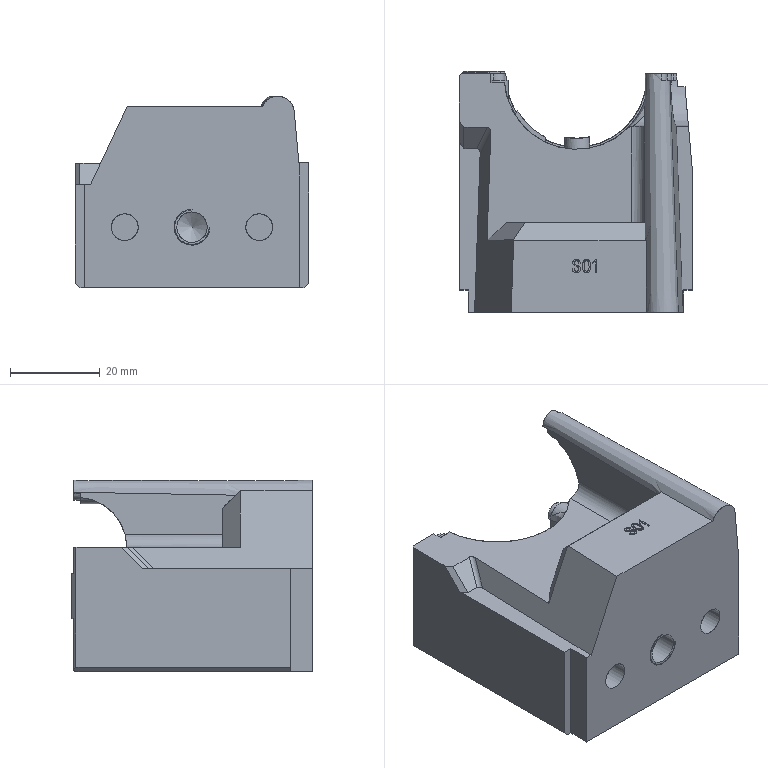NC program | PowerMill | posted with a generic post | part box 52 x 53.756 x 42.711 mm
Whole program:
%
O0001
N104 ( POWERMILL CB  : 2026004.0)
N105 ( POST VER      : 2026.0.0.5161)
N106 ( OPTION FILE   : FANUC)
N107 ( OUTPUT WORKPLANE : 1)
N108 (  )
N109 ( TOOL LIST )
N110 (--------------------------------)
N111 ( NO. | ID | DIA.| TIP RAD|LENGTH)
N112 (--------------------------------)
N113 (    1|D8_3| 8.0 |  0.0   | 99.0 )
N114 (--------------------------------)
N115 (  )
N116 ( NUMBER OF TOOLPATHS: 2.0 )
N117 ( ESTIMATED PROGRAM DURATION: 0 HOURS 2 MIN 27 SEC)
N118 (  )
N119 G00 G21 G80 G40 G17
N120 G90
N121 G54
N122 G53 Z0.0
N123 (---------------)
N124 ( START TOOLPATH : 04精光-D8-偏置平坦面 )
N125 (---------------)
N126 ( TOOL NO.    :1 )
N127 ( TOOL TYPE   : ENDMILL)
N128 ( TOOL ID     : D8_3)
N129 ( TOOL DIA    : 8.0 LENGTH 99.0)
N130 T1
N131 M6
N132 S3500 M03
N133 G00 G90 X-27.783 Y-7.9491
N134 G43 Z20.0 H1
N135
N136 G05 P10000 R8
N137 Z-2.0
N138 G01 Z-5.0 F480.0
N139 X-26.3387 Y-3.984 F800.0
N140 G03 X-26.0 Y-3.9983 I0.3387 J3.9841
N141 G01 X-25.2845
N142 G02 X-28.1881 Y-0.3178 I1.2821 J3.997
N143 G02 X-28.2001 Y0.2956 I6.337 J0.4306
N144 G01 Y44.8679
N145 G02 X-27.9783 Y46.1846 I4.0947 J-0.0127
N146 G00 Z5.0625
N147 G01 X33.9831 Y-1.6873 F10000.0
N148 G00 Z-2.0
N149 G01 Z-5.0 F480.0
N150 X29.9838 Y-0.3406 F800.0
N151 G03 X29.9983 Y0.0 I-3.9839 J0.3406
N152 G01 Y42.71
N153 G03 X27.9782 Y46.1846 I-3.9983 J0.0
N154 G02 X28.2001 Y44.8679 I-3.8786 J-1.3304
N155 G01 Y0.2956
N156 G02 X28.1333 Y-0.7465 I-4.9114 J-0.2084
N157 G02 X25.2845 Y-3.9983 I-4.1307 J0.7449
N158 G00 Z20.0
N159 G05 P0
N160 (---------------)
N161 ( END TOOLPATH : 04精光-D8-偏置平坦面 )
N162 (---------------)
N163 ( START TOOLPATH : 03精光-D8-等高 )
N164 (---------------)
N165 S5500 M03
N166 G00 X28.2044 Y43.463 Z20.0
N167 G05 P10000 R8
N168 Z2.9018
N169 G01 Z-0.0982 F1200.0
N170 G03 X27.99 Y42.663 I1.3856 J-0.8 F2000.0
N171 G01 Y0.047
N172 G03 X28.2044 Y-0.753 I1.6 J0.0
N173 G01 X28.2217 Y-0.7831 Z-0.1125
N174 X28.2289 Y-0.7955 Z-0.1472
N175 X28.2217 Y-0.7831 Z-0.1819
N176 X28.2044 Y-0.753 Z-0.1963
N177 G02 X27.99 Y0.047 I1.3856 J0.8
N178 G01 Y42.663
N179 G02 X28.2044 Y43.463 I1.6 J0.0
N180 G01 X28.2217 Y43.4931 Z-0.2107
N181 X28.2289 Y43.5055 Z-0.2454
N182 X28.2217 Y43.4931 Z-0.2801
N183 X28.2044 Y43.463 Z-0.2945
N184 G03 X27.99 Y42.663 I1.3856 J-0.8
N185 G01 Y0.047
N186 G03 X28.2044 Y-0.753 I1.6 J0.0
N187 G01 X28.2217 Y-0.7831 Z-0.3088
N188 X28.2289 Y-0.7955 Z-0.3435
N189 X28.2217 Y-0.7831 Z-0.3783
N190 X28.2044 Y-0.753 Z-0.3926
N191 G02 X27.99 Y0.047 I1.3856 J0.8
N192 G01 Y42.663
N193 G02 X28.2044 Y43.463 I1.6 J0.0
N194 G01 X28.2217 Y43.4931 Z-0.407
N195 X28.2289 Y43.5055 Z-0.4417
N196 X28.2217 Y43.4931 Z-0.4764
N197 X28.2044 Y43.463 Z-0.4908
N198 G03 X27.99 Y42.663 I1.3856 J-0.8
N199 G01 Y0.047
N200 G03 X28.2044 Y-0.753 I1.6 J0.0
N201 G01 X28.2217 Y-0.7831 Z-0.5052
N202 X28.2289 Y-0.7955 Z-0.5399
N203 X28.2217 Y-0.7831 Z-0.5746
N204 X28.2044 Y-0.753 Z-0.5889
N205 G02 X27.99 Y0.047 I1.3856 J0.8
N206 G01 Y42.663
N207 G02 X28.2044 Y43.463 I1.6 J0.0
N208 G01 X28.2217 Y43.4931 Z-0.6033
N209 X28.2289 Y43.5055 Z-0.638
N210 X28.2217 Y43.4931 Z-0.6727
N211 X28.2044 Y43.463 Z-0.6871
N212 G03 X27.99 Y42.663 I1.3856 J-0.8
N213 G01 Y0.047
N214 G03 X28.2044 Y-0.753 I1.6 J0.0
N215 G01 X28.2217 Y-0.7831 Z-0.7015
N216 X28.2289 Y-0.7955 Z-0.7362
N217 X28.2217 Y-0.7831 Z-0.7709
N218 X28.2044 Y-0.753 Z-0.7853
N219 G02 X27.99 Y0.047 I1.3856 J0.8
N220 G01 Y42.663
N221 G02 X28.2044 Y43.463 I1.6 J0.0
N222 G01 X28.2217 Y43.4931 Z-0.7996
N223 X28.2289 Y43.5055 Z-0.8343
N224 X28.2217 Y43.4931 Z-0.869
N225 X28.2044 Y43.463 Z-0.8834
N226 G03 X27.99 Y42.663 I1.3856 J-0.8
N227 G01 Y0.047
N228 G03 X28.2044 Y-0.753 I1.6 J0.0
N229 G01 X28.2217 Y-0.7831 Z-0.8978
N230 X28.2289 Y-0.7955 Z-0.9325
N231 X28.2217 Y-0.7831 Z-0.9672
N232 X28.2044 Y-0.753 Z-0.9816
N233 G02 X27.99 Y0.047 I1.3856 J0.8
N234 G01 Y42.663
N235 G02 X28.2044 Y43.463 I1.6 J0.0
N236 G01 X28.2217 Y43.4931 Z-0.9959
N237 X28.2289 Y43.5055 Z-1.0306
N238 X28.2217 Y43.4931 Z-1.0654
N239 X28.2044 Y43.463 Z-1.0797
N240 G03 X27.99 Y42.663 I1.3856 J-0.8
N241 G01 Y0.047
N242 G03 X28.2044 Y-0.753 I1.6 J0.0
N243 G01 X28.2217 Y-0.7831 Z-1.0941
N244 X28.2289 Y-0.7955 Z-1.1288
N245 X28.2217 Y-0.7831 Z-1.1635
N246 X28.2044 Y-0.753 Z-1.1779
N247 G02 X27.99 Y0.047 I1.3856 J0.8
N248 G01 Y42.663
N249 G02 X28.2044 Y43.463 I1.6 J0.0
N250 G01 X28.2217 Y43.4931 Z-1.1923
N251 X28.2289 Y43.5055 Z-1.227
N252 X28.2217 Y43.4931 Z-1.2617
N253 X28.2044 Y43.463 Z-1.276
N254 G03 X27.99 Y42.663 I1.3856 J-0.8
N255 G01 Y0.047
N256 G03 X28.2044 Y-0.753 I1.6 J0.0
N257 G01 X28.2217 Y-0.7831 Z-1.2904
N258 X28.2289 Y-0.7955 Z-1.3251
N259 X28.2217 Y-0.7831 Z-1.3598
N260 X28.2044 Y-0.753 Z-1.3742
N261 G02 X27.99 Y0.047 I1.3856 J0.8
N262 G01 Y42.663
N263 G02 X28.2044 Y43.463 I1.6 J0.0
N264 G01 X28.2217 Y43.4931 Z-1.3886
N265 X28.2289 Y43.5055 Z-1.4233
N266 X28.2217 Y43.4931 Z-1.458
N267 X28.2044 Y43.463 Z-1.4724
N268 G03 X27.99 Y42.663 I1.3856 J-0.8
N269 G01 Y0.047
N270 G03 X28.2044 Y-0.753 I1.6 J0.0
N271 G01 X28.2217 Y-0.7831 Z-1.4867
N272 X28.2289 Y-0.7955 Z-1.5214
N273 X28.2217 Y-0.7831 Z-1.5561
N274 X28.2044 Y-0.753 Z-1.5705
N275 G02 X27.99 Y0.047 I1.3856 J0.8
N276 G01 Y42.663
N277 G02 X28.2044 Y43.463 I1.6 J0.0
N278 G01 X28.2217 Y43.4931 Z-1.5849
N279 X28.2289 Y43.5055 Z-1.6196
N280 X28.2217 Y43.4931 Z-1.6543
N281 X28.2044 Y43.463 Z-1.6687
N282 G03 X27.99 Y42.663 I1.3856 J-0.8
N283 G01 Y0.047
N284 G03 X28.2044 Y-0.753 I1.6 J0.0
N285 G01 X28.2217 Y-0.7831 Z-1.683
N286 X28.2289 Y-0.7955 Z-1.7177
N287 X28.2217 Y-0.7831 Z-1.7524
N288 X28.2044 Y-0.753 Z-1.7668
N289 G02 X27.99 Y0.047 I1.3856 J0.8
N290 G01 Y42.663
N291 G02 X28.2044 Y43.463 I1.6 J0.0
N292 G01 X28.2217 Y43.4931 Z-1.7812
N293 X28.2289 Y43.5055 Z-1.8159
N294 X28.2217 Y43.4931 Z-1.8506
N295 X28.2044 Y43.463 Z-1.865
N296 G03 X27.99 Y42.663 I1.3856 J-0.8
N297 G01 Y0.047
N298 G03 X28.2044 Y-0.753 I1.6 J0.0
N299 G01 X28.2217 Y-0.7831 Z-1.8794
N300 X28.2289 Y-0.7955 Z-1.9141
N301 X28.2217 Y-0.7831 Z-1.9488
N302 X28.2044 Y-0.753 Z-1.9631
N303 G02 X27.99 Y0.047 I1.3856 J0.8
N304 G01 Y42.663
N305 G02 X28.2044 Y43.463 I1.6 J0.0
N306 G01 X28.2217 Y43.4931 Z-1.9775
N307 X28.2289 Y43.5055 Z-2.0122
N308 X28.2217 Y43.4931 Z-2.0469
N309 X28.2044 Y43.463 Z-2.0613
N310 G03 X27.99 Y42.663 I1.3856 J-0.8
N311 G01 Y0.047
N312 G03 X28.2044 Y-0.753 I1.6 J0.0
N313 G01 X28.2217 Y-0.7831 Z-2.0757
N314 X28.2289 Y-0.7955 Z-2.1104
N315 X28.2217 Y-0.7831 Z-2.1451
N316 X28.2044 Y-0.753 Z-2.1595
N317 G02 X27.99 Y0.047 I1.3856 J0.8
N318 G01 Y42.663
N319 G02 X28.2044 Y43.463 I1.6 J0.0
N320 G01 X28.2217 Y43.4931 Z-2.1738
N321 X28.2289 Y43.5055 Z-2.2085
N322 X28.2217 Y43.4931 Z-2.2432
N323 X28.2044 Y43.463 Z-2.2576
N324 G03 X27.99 Y42.663 I1.3856 J-0.8
N325 G01 Y0.047
N326 G03 X28.2044 Y-0.753 I1.6 J0.0
N327 G01 X28.2217 Y-0.7831 Z-2.272
N328 X28.2289 Y-0.7955 Z-2.3067
N329 X28.2217 Y-0.7831 Z-2.3414
N330 X28.2044 Y-0.753 Z-2.3558
N331 G02 X27.99 Y0.047 I1.3856 J0.8
N332 G01 Y42.663
N333 G02 X28.2044 Y43.463 I1.6 J0.0
N334 G01 X28.2217 Y43.4931 Z-2.3701
N335 X28.2289 Y43.5055 Z-2.4048
N336 X28.2217 Y43.4931 Z-2.4395
N337 X28.2044 Y43.463 Z-2.4539
N338 G03 X27.99 Y42.663 I1.3856 J-0.8
N339 G01 Y0.047
N340 G03 X28.2044 Y-0.753 I1.6 J0.0
N341 G01 X28.2217 Y-0.7831 Z-2.4683
N342 X28.2289 Y-0.7955 Z-2.503
N343 X28.2217 Y-0.7831 Z-2.5377
N344 X28.2044 Y-0.753 Z-2.5521
N345 G02 X27.99 Y0.047 I1.3856 J0.8
N346 G01 Y42.663
N347 G02 X28.2044 Y43.463 I1.6 J0.0
N348 G01 X28.2217 Y43.4931 Z-2.5665
N349 X28.2289 Y43.5055 Z-2.6012
N350 X28.2217 Y43.4931 Z-2.6359
N351 X28.2044 Y43.463 Z-2.6502
N352 G03 X27.99 Y42.663 I1.3856 J-0.8
N353 G01 Y0.047
N354 G03 X28.2044 Y-0.753 I1.6 J0.0
N355 G01 X28.2217 Y-0.7831 Z-2.6646
N356 X28.2289 Y-0.7955 Z-2.6993
N357 X28.2217 Y-0.7831 Z-2.734
N358 X28.2044 Y-0.753 Z-2.7484
N359 G02 X27.99 Y0.047 I1.3856 J0.8
N360 G01 Y42.663
N361 G02 X28.2044 Y43.463 I1.6 J0.0
N362 G01 X28.2217 Y43.4931 Z-2.7628
N363 X28.2289 Y43.5055 Z-2.7975
N364 X28.2217 Y43.4931 Z-2.8322
N365 X28.2044 Y43.463 Z-2.8465
N366 G03 X27.99 Y42.663 I1.3856 J-0.8
N367 G01 Y0.047
N368 G03 X28.2044 Y-0.753 I1.6 J0.0
N369 G01 X28.2217 Y-0.7831 Z-2.8609
N370 X28.2289 Y-0.7955 Z-2.8956
N371 X28.2217 Y-0.7831 Z-2.9303
N372 X28.2044 Y-0.753 Z-2.9447
N373 G02 X27.99 Y0.047 I1.3856 J0.8
N374 G01 Y42.663
N375 G02 X28.2044 Y43.463 I1.6 J0.0
N376 G01 X28.2217 Y43.4931 Z-2.9591
N377 X28.2289 Y43.5055 Z-2.9938
N378 X28.2217 Y43.4931 Z-3.0285
N379 X28.2044 Y43.463 Z-3.0429
N380 G03 X27.99 Y42.663 I1.3856 J-0.8
N381 G01 Y0.047
N382 G03 X28.2044 Y-0.753 I1.6 J0.0
N383 G01 X28.2217 Y-0.7831 Z-3.0572
N384 X28.2289 Y-0.7955 Z-3.0919
N385 X28.2217 Y-0.7831 Z-3.1266
N386 X28.2044 Y-0.753 Z-3.141
N387 G02 X27.99 Y0.047 I1.3856 J0.8
N388 G01 Y42.663
N389 G02 X28.2044 Y43.463 I1.6 J0.0
N390 G01 X28.2217 Y43.4931 Z-3.1554
N391 X28.2289 Y43.5055 Z-3.1901
N392 X28.2217 Y43.4931 Z-3.2248
N393 X28.2044 Y43.463 Z-3.2392
N394 G03 X27.99 Y42.663 I1.3856 J-0.8
N395 G01 Y0.047
N396 G03 X28.2044 Y-0.753 I1.6 J0.0
N397 G01 X28.2217 Y-0.7831 Z-3.2536
N398 X28.2289 Y-0.7955 Z-3.2883
N399 X28.2217 Y-0.7831 Z-3.323
N400 X28.2044 Y-0.753 Z-3.3373
N401 G02 X27.99 Y0.047 I1.3856 J0.8
N402 G01 Y42.663
N403 G02 X28.2044 Y43.463 I1.6 J0.0
N404 G01 X28.2217 Y43.4931 Z-3.3517
N405 X28.2289 Y43.5055 Z-3.3864
N406 X28.2217 Y43.4931 Z-3.4211
N407 X28.2044 Y43.463 Z-3.4355
N408 G03 X27.99 Y42.663 I1.3856 J-0.8
N409 G01 Y0.047
N410 G03 X28.2044 Y-0.753 I1.6 J0.0
N411 G01 X28.2217 Y-0.7831 Z-3.4499
N412 X28.2289 Y-0.7955 Z-3.4846
N413 X28.2217 Y-0.7831 Z-3.5193
N414 X28.2044 Y-0.753 Z-3.5336
N415 G02 X27.99 Y0.047 I1.3856 J0.8
N416 G01 Y42.663
N417 G02 X28.2044 Y43.463 I1.6 J0.0
N418 G01 X28.2217 Y43.4931 Z-3.548
N419 X28.2289 Y43.5055 Z-3.5827
N420 X28.2217 Y43.4931 Z-3.6174
N421 X28.2044 Y43.463 Z-3.6318
N422 G03 X27.99 Y42.663 I1.3856 J-0.8
N423 G01 Y0.047
N424 G03 X28.2044 Y-0.753 I1.6 J0.0
N425 G01 X28.2217 Y-0.7831 Z-3.6462
N426 X28.2289 Y-0.7955 Z-3.6809
N427 X28.2217 Y-0.7831 Z-3.7156
N428 X28.2044 Y-0.753 Z-3.73
N429 G02 X27.99 Y0.047 I1.3856 J0.8
N430 G01 Y42.663
N431 G02 X28.2044 Y43.463 I1.6 J0.0
N432 G01 X28.2217 Y43.4931 Z-3.7443
N433 X28.2289 Y43.5055 Z-3.779
N434 X28.2217 Y43.4931 Z-3.8137
N435 X28.2044 Y43.463 Z-3.8281
N436 G03 X27.99 Y42.663 I1.3856 J-0.8
N437 G01 Y0.047
N438 G03 X28.2044 Y-0.753 I1.6 J0.0
N439 G01 X28.2217 Y-0.7831 Z-3.8425
N440 X28.2289 Y-0.7955 Z-3.8772
N441 X28.2217 Y-0.7831 Z-3.9119
N442 X28.2044 Y-0.753 Z-3.9263
N443 G02 X27.99 Y0.047 I1.3856 J0.8
N444 G01 Y42.663
N445 G02 X28.2044 Y43.463 I1.6 J0.0
N446 G01 X28.2217 Y43.4931 Z-3.9406
N447 X28.2289 Y43.5055 Z-3.9754
N448 X28.2217 Y43.4931 Z-4.0101
N449 X28.2044 Y43.463 Z-4.0244
N450 G03 X27.99 Y42.663 I1.3856 J-0.8
N451 G01 Y0.047
N452 G03 X28.2044 Y-0.753 I1.6 J0.0
N453 G01 X28.2217 Y-0.7831 Z-4.0388
N454 X28.2289 Y-0.7955 Z-4.0735
N455 X28.2217 Y-0.7831 Z-4.1082
N456 X28.2044 Y-0.753 Z-4.1226
N457 G02 X27.99 Y0.047 I1.3856 J0.8
N458 G01 Y42.663
N459 G02 X28.2044 Y43.463 I1.6 J0.0
N460 G01 X28.2217 Y43.4931 Z-4.137
N461 X28.2289 Y43.5055 Z-4.1717
N462 X28.2217 Y43.4931 Z-4.2064
N463 X28.2044 Y43.463 Z-4.2207
N464 G03 X27.99 Y42.663 I1.3856 J-0.8
N465 G01 Y0.047
N466 G03 X28.2044 Y-0.753 I1.6 J0.0
N467 G01 X28.2217 Y-0.7831 Z-4.2351
N468 X28.2289 Y-0.7955 Z-4.2698
N469 X28.2217 Y-0.7831 Z-4.3045
N470 X28.2044 Y-0.753 Z-4.3189
N471 G02 X27.99 Y0.047 I1.3856 J0.8
N472 G01 Y42.663
N473 G02 X28.2044 Y43.463 I1.6 J0.0
N474 G01 X28.2217 Y43.4931 Z-4.3333
N475 X28.2289 Y43.5055 Z-4.368
N476 X28.2217 Y43.4931 Z-4.4027
N477 X28.2044 Y43.463 Z-4.4171
N478 G03 X27.99 Y42.663 I1.3856 J-0.8
N479 G01 Y0.047
N480 G03 X28.2044 Y-0.753 I1.6 J0.0
N481 G01 X28.2217 Y-0.7831 Z-4.4314
N482 X28.2289 Y-0.7955 Z-4.4661
N483 X28.2217 Y-0.7831 Z-4.5008
N484 X28.2044 Y-0.753 Z-4.5152
N485 G02 X27.99 Y0.047 I1.3856 J0.8
N486 G01 Y42.663
N487 G02 X28.2044 Y43.463 I1.6 J0.0
N488 G01 X28.2217 Y43.4931 Z-4.5296
N489 X28.2289 Y43.5055 Z-4.5643
N490 X28.2217 Y43.4931 Z-4.599
N491 X28.2044 Y43.463 Z-4.6134
N492 G03 X27.99 Y42.663 I1.3856 J-0.8
N493 G01 Y0.047
N494 G03 X28.2044 Y-0.753 I1.6 J0.0
N495 G01 X28.2217 Y-0.7831 Z-4.6277
N496 X28.2289 Y-0.7955 Z-4.6625
N497 X28.2217 Y-0.7831 Z-4.6972
N498 X28.2044 Y-0.753 Z-4.7115
N499 G02 X27.99 Y0.047 I1.3856 J0.8
N500 G01 Y42.663
N501 G02 X28.2044 Y43.463 I1.6 J0.0
N502 G01 X28.2217 Y43.4931 Z-4.7259
N503 X28.2289 Y43.5055 Z-4.7606
N504 X28.2217 Y43.4931 Z-4.7953
N505 X28.2044 Y43.463 Z-4.8097
N506 G03 X27.99 Y42.663 I1.3856 J-0.8
N507 G01 Y0.047
N508 G03 X28.2044 Y-0.753 I1.6 J0.0
N509 G01 X28.2217 Y-0.7831 Z-4.8241
N510 X28.2289 Y-0.7955 Z-4.8588
N511 X28.2217 Y-0.7831 Z-4.8935
N512 X28.2044 Y-0.753 Z-4.9078
N513 G02 X27.99 Y0.047 I1.3856 J0.8
N514 G01 Y42.663
N515 G02 X28.2044 Y43.463 I1.6 J0.0
N516 G00 Z5.0391
N517 G01 X-28.2044 Y-0.753 F10000.0
N518 G00 Z2.9018
N519 G01 Z-0.0982 F1200.0
N520 G03 X-27.99 Y0.047 I-1.3856 J0.8 F2000.0
N521 G01 Y42.663
N522 G03 X-28.2044 Y43.463 I-1.6 J0.0
N523 G01 X-28.2217 Y43.4931 Z-0.1125
N524 X-28.2289 Y43.5055 Z-0.1472
N525 X-28.2217 Y43.4931 Z-0.1819
N526 X-28.2044 Y43.463 Z-0.1963
N527 G02 X-27.99 Y42.663 I-1.3856 J-0.8
N528 G01 Y0.047
N529 G02 X-28.2044 Y-0.753 I-1.6 J0.0
N530 G01 X-28.2217 Y-0.7831 Z-0.2107
N531 X-28.2289 Y-0.7955 Z-0.2454
N532 X-28.2217 Y-0.7831 Z-0.2801
N533 X-28.2044 Y-0.753 Z-0.2945
N534 G03 X-27.99 Y0.047 I-1.3856 J0.8
N535 G01 Y42.663
N536 G03 X-28.2044 Y43.463 I-1.6 J0.0
N537 G01 X-28.2217 Y43.4931 Z-0.3088
N538 X-28.2289 Y43.5055 Z-0.3435
N539 X-28.2217 Y43.4931 Z-0.3783
N540 X-28.2044 Y43.463 Z-0.3926
N541 G02 X-27.99 Y42.663 I-1.3856 J-0.8
N542 G01 Y0.047
N543 G02 X-28.2044 Y-0.753 I-1.6 J0.0
N544 G01 X-28.2217 Y-0.7831 Z-0.407
N545 X-28.2289 Y-0.7955 Z-0.4417
N546 X-28.2217 Y-0.7831 Z-0.4764
N547 X-28.2044 Y-0.753 Z-0.4908
N548 G03 X-27.99 Y0.047 I-1.3856 J0.8
N549 G01 Y42.663
N550 G03 X-28.2044 Y43.463 I-1.6 J0.0
N551 G01 X-28.2217 Y43.4931 Z-0.5052
N552 X-28.2289 Y43.5055 Z-0.5399
N553 X-28.2217 Y43.4931 Z-0.5746
N554 X-28.2044 Y43.463 Z-0.5889
N555 G02 X-27.99 Y42.663 I-1.3856 J-0.8
N556 G01 Y0.047
N557 G02 X-28.2044 Y-0.753 I-1.6 J0.0
N558 G01 X-28.2217 Y-0.7831 Z-0.6033
N559 X-28.2289 Y-0.7955 Z-0.638
N560 X-28.2217 Y-0.7831 Z-0.6727
N561 X-28.2044 Y-0.753 Z-0.6871
N562 G03 X-27.99 Y0.047 I-1.3856 J0.8
N563 G01 Y42.663
N564 G03 X-28.2044 Y43.463 I-1.6 J0.0
N565 G01 X-28.2217 Y43.4931 Z-0.7015
N566 X-28.2289 Y43.5055 Z-0.7362
N567 X-28.2217 Y43.4931 Z-0.7709
N568 X-28.2044 Y43.463 Z-0.7853
N569 G02 X-27.99 Y42.663 I-1.3856 J-0.8
N570 G01 Y0.047
N571 G02 X-28.2044 Y-0.753 I-1.6 J0.0
N572 G01 X-28.2217 Y-0.7831 Z-0.7996
N573 X-28.2289 Y-0.7955 Z-0.8343
N574 X-28.2217 Y-0.7831 Z-0.869
N575 X-28.2044 Y-0.753 Z-0.8834
N576 G03 X-27.99 Y0.047 I-1.3856 J0.8
N577 G01 Y42.663
N578 G03 X-28.2044 Y43.463 I-1.6 J0.0
N579 G01 X-28.2217 Y43.4931 Z-0.8978
N580 X-28.2289 Y43.5055 Z-0.9325
N581 X-28.2217 Y43.4931 Z-0.9672
N582 X-28.2044 Y43.463 Z-0.9816
N583 G02 X-27.99 Y42.663 I-1.3856 J-0.8
N584 G01 Y0.047
N585 G02 X-28.2044 Y-0.753 I-1.6 J0.0
N586 G01 X-28.2217 Y-0.7831 Z-0.9959
N587 X-28.2289 Y-0.7955 Z-1.0306
N588 X-28.2217 Y-0.7831 Z-1.0654
N589 X-28.2044 Y-0.753 Z-1.0797
N590 G03 X-27.99 Y0.047 I-1.3856 J0.8
N591 G01 Y42.663
N592 G03 X-28.2044 Y43.463 I-1.6 J0.0
N593 G01 X-28.2217 Y43.4931 Z-1.0941
N594 X-28.2289 Y43.5055 Z-1.1288
N595 X-28.2217 Y43.4931 Z-1.1635
N596 X-28.2044 Y43.463 Z-1.1779
N597 G02 X-27.99 Y42.663 I-1.3856 J-0.8
N598 G01 Y0.047
N599 G02 X-28.2044 Y-0.753 I-1.6 J0.0
N600 G01 X-28.2217 Y-0.7831 Z-1.1923
N601 X-28.2289 Y-0.7955 Z-1.227
N602 X-28.2217 Y-0.7831 Z-1.2617
N603 X-28.2044 Y-0.753 Z-1.276
N604 G03 X-27.99 Y0.047 I-1.3856 J0.8
N605 G01 Y42.663
N606 G03 X-28.2044 Y43.463 I-1.6 J0.0
N607 G01 X-28.2217 Y43.4931 Z-1.2904
N608 X-28.2289 Y43.5055 Z-1.3251
N609 X-28.2217 Y43.4931 Z-1.3598
N610 X-28.2044 Y43.463 Z-1.3742
N611 G02 X-27.99 Y42.663 I-1.3856 J-0.8
N612 G01 Y0.047
N613 G02 X-28.2044 Y-0.753 I-1.6 J0.0
N614 G01 X-28.2217 Y-0.7831 Z-1.3886
N615 X-28.2289 Y-0.7955 Z-1.4233
N616 X-28.2217 Y-0.7831 Z-1.458
N617 X-28.2044 Y-0.753 Z-1.4724
N618 G03 X-27.99 Y0.047 I-1.3856 J0.8
N619 G01 Y42.663
N620 G03 X-28.2044 Y43.463 I-1.6 J0.0
N621 G01 X-28.2217 Y43.4931 Z-1.4867
N622 X-28.2289 Y43.5055 Z-1.5214
N623 X-28.2217 Y43.4931 Z-1.5561
N624 X-28.2044 Y43.463 Z-1.5705
N625 G02 X-27.99 Y42.663 I-1.3856 J-0.8
N626 G01 Y0.047
N627 G02 X-28.2044 Y-0.753 I-1.6 J0.0
N628 G01 X-28.2217 Y-0.7831 Z-1.5849
N629 X-28.2289 Y-0.7955 Z-1.6196
N630 X-28.2217 Y-0.7831 Z-1.6543
N631 X-28.2044 Y-0.753 Z-1.6687
N632 G03 X-27.99 Y0.047 I-1.3856 J0.8
N633 G01 Y42.663
N634 G03 X-28.2044 Y43.463 I-1.6 J0.0
N635 G01 X-28.2217 Y43.4931 Z-1.683
N636 X-28.2289 Y43.5055 Z-1.7177
N637 X-28.2217 Y43.4931 Z-1.7524
N638 X-28.2044 Y43.463 Z-1.7668
N639 G02 X-27.99 Y42.663 I-1.3856 J-0.8
N640 G01 Y0.047
N641 G02 X-28.2044 Y-0.753 I-1.6 J0.0
N642 G01 X-28.2217 Y-0.7831 Z-1.7812
N643 X-28.2289 Y-0.7955 Z-1.8159
N644 X-28.2217 Y-0.7831 Z-1.8506
N645 X-28.2044 Y-0.753 Z-1.865
N646 G03 X-27.99 Y0.047 I-1.3856 J0.8
N647 G01 Y42.663
N648 G03 X-28.2044 Y43.463 I-1.6 J0.0
N649 G01 X-28.2217 Y43.4931 Z-1.8794
N650 X-28.2289 Y43.5055 Z-1.9141
N651 X-28.2217 Y43.4931 Z-1.9488
N652 X-28.2044 Y43.463 Z-1.9631
N653 G02 X-27.99 Y42.663 I-1.3856 J-0.8
N654 G01 Y0.047
N655 G02 X-28.2044 Y-0.753 I-1.6 J0.0
N656 G01 X-28.2217 Y-0.7831 Z-1.9775
N657 X-28.2289 Y-0.7955 Z-2.0122
N658 X-28.2217 Y-0.7831 Z-2.0469
N659 X-28.2044 Y-0.753 Z-2.0613
N660 G03 X-27.99 Y0.047 I-1.3856 J0.8
N661 G01 Y42.663
N662 G03 X-28.2044 Y43.463 I-1.6 J0.0
N663 G01 X-28.2217 Y43.4931 Z-2.0757
N664 X-28.2289 Y43.5055 Z-2.1104
N665 X-28.2217 Y43.4931 Z-2.1451
N666 X-28.2044 Y43.463 Z-2.1595
N667 G02 X-27.99 Y42.663 I-1.3856 J-0.8
N668 G01 Y0.047
N669 G02 X-28.2044 Y-0.753 I-1.6 J0.0
N670 G01 X-28.2217 Y-0.7831 Z-2.1738
N671 X-28.2289 Y-0.7955 Z-2.2085
N672 X-28.2217 Y-0.7831 Z-2.2432
N673 X-28.2044 Y-0.753 Z-2.2576
N674 G03 X-27.99 Y0.047 I-1.3856 J0.8
N675 G01 Y42.663
N676 G03 X-28.2044 Y43.463 I-1.6 J0.0
N677 G01 X-28.2217 Y43.4931 Z-2.272
N678 X-28.2289 Y43.5055 Z-2.3067
N679 X-28.2217 Y43.4931 Z-2.3414
N680 X-28.2044 Y43.463 Z-2.3558
N681 G02 X-27.99 Y42.663 I-1.3856 J-0.8
N682 G01 Y0.047
N683 G02 X-28.2044 Y-0.753 I-1.6 J0.0
N684 G01 X-28.2217 Y-0.7831 Z-2.3701
N685 X-28.2289 Y-0.7955 Z-2.4048
N686 X-28.2217 Y-0.7831 Z-2.4395
N687 X-28.2044 Y-0.753 Z-2.4539
N688 G03 X-27.99 Y0.047 I-1.3856 J0.8
N689 G01 Y42.663
N690 G03 X-28.2044 Y43.463 I-1.6 J0.0
N691 G01 X-28.2217 Y43.4931 Z-2.4683
N692 X-28.2289 Y43.5055 Z-2.503
N693 X-28.2217 Y43.4931 Z-2.5377
N694 X-28.2044 Y43.463 Z-2.5521
N695 G02 X-27.99 Y42.663 I-1.3856 J-0.8
N696 G01 Y0.047
N697 G02 X-28.2044 Y-0.753 I-1.6 J0.0
N698 G01 X-28.2217 Y-0.7831 Z-2.5665
N699 X-28.2289 Y-0.7955 Z-2.6012
N700 X-28.2217 Y-0.7831 Z-2.6359
N701 X-28.2044 Y-0.753 Z-2.6502
N702 G03 X-27.99 Y0.047 I-1.3856 J0.8
N703 G01 Y42.663
N704 G03 X-28.2044 Y43.463 I-1.6 J0.0
N705 G01 X-28.2217 Y43.4931 Z-2.6646
N706 X-28.2289 Y43.5055 Z-2.6993
N707 X-28.2217 Y43.4931 Z-2.734
N708 X-28.2044 Y43.463 Z-2.7484
N709 G02 X-27.99 Y42.663 I-1.3856 J-0.8
N710 G01 Y0.047
N711 G02 X-28.2044 Y-0.753 I-1.6 J0.0
N712 G01 X-28.2217 Y-0.7831 Z-2.7628
N713 X-28.2289 Y-0.7955 Z-2.7975
N714 X-28.2217 Y-0.7831 Z-2.8322
N715 X-28.2044 Y-0.753 Z-2.8465
N716 G03 X-27.99 Y0.047 I-1.3856 J0.8
N717 G01 Y42.663
N718 G03 X-28.2044 Y43.463 I-1.6 J0.0
N719 G01 X-28.2217 Y43.4931 Z-2.8609
N720 X-28.2289 Y43.5055 Z-2.8956
N721 X-28.2217 Y43.4931 Z-2.9303
N722 X-28.2044 Y43.463 Z-2.9447
N723 G02 X-27.99 Y42.663 I-1.3856 J-0.8
N724 G01 Y0.047
N725 G02 X-28.2044 Y-0.753 I-1.6 J0.0
N726 G01 X-28.2217 Y-0.7831 Z-2.9591
N727 X-28.2289 Y-0.7955 Z-2.9938
N728 X-28.2217 Y-0.7831 Z-3.0285
N729 X-28.2044 Y-0.753 Z-3.0429
N730 G03 X-27.99 Y0.047 I-1.3856 J0.8
N731 G01 Y42.663
N732 G03 X-28.2044 Y43.463 I-1.6 J0.0
N733 G01 X-28.2217 Y43.4931 Z-3.0572
N734 X-28.2289 Y43.5055 Z-3.0919
N735 X-28.2217 Y43.4931 Z-3.1266
N736 X-28.2044 Y43.463 Z-3.141
N737 G02 X-27.99 Y42.663 I-1.3856 J-0.8
N738 G01 Y0.047
N739 G02 X-28.2044 Y-0.753 I-1.6 J0.0
N740 G01 X-28.2217 Y-0.7831 Z-3.1554
N741 X-28.2289 Y-0.7955 Z-3.1901
N742 X-28.2217 Y-0.7831 Z-3.2248
N743 X-28.2044 Y-0.753 Z-3.2392
N744 G03 X-27.99 Y0.047 I-1.3856 J0.8
N745 G01 Y42.663
N746 G03 X-28.2044 Y43.463 I-1.6 J0.0
N747 G01 X-28.2217 Y43.4931 Z-3.2536
N748 X-28.2289 Y43.5055 Z-3.2883
N749 X-28.2217 Y43.4931 Z-3.323
N750 X-28.2044 Y43.463 Z-3.3373
N751 G02 X-27.99 Y42.663 I-1.3856 J-0.8
N752 G01 Y0.047
N753 G02 X-28.2044 Y-0.753 I-1.6 J0.0
N754 G01 X-28.2217 Y-0.7831 Z-3.3517
N755 X-28.2289 Y-0.7955 Z-3.3864
N756 X-28.2217 Y-0.7831 Z-3.4211
N757 X-28.2044 Y-0.753 Z-3.4355
N758 G03 X-27.99 Y0.047 I-1.3856 J0.8
N759 G01 Y42.663
N760 G03 X-28.2044 Y43.463 I-1.6 J0.0
N761 G01 X-28.2217 Y43.4931 Z-3.4499
N762 X-28.2289 Y43.5055 Z-3.4846
N763 X-28.2217 Y43.4931 Z-3.5193
N764 X-28.2044 Y43.463 Z-3.5336
N765 G02 X-27.99 Y42.663 I-1.3856 J-0.8
N766 G01 Y0.047
N767 G02 X-28.2044 Y-0.753 I-1.6 J0.0
N768 G01 X-28.2217 Y-0.7831 Z-3.548
N769 X-28.2289 Y-0.7955 Z-3.5827
N770 X-28.2217 Y-0.7831 Z-3.6174
N771 X-28.2044 Y-0.753 Z-3.6318
N772 G03 X-27.99 Y0.047 I-1.3856 J0.8
N773 G01 Y42.663
N774 G03 X-28.2044 Y43.463 I-1.6 J0.0
N775 G01 X-28.2217 Y43.4931 Z-3.6462
N776 X-28.2289 Y43.5055 Z-3.6809
N777 X-28.2217 Y43.4931 Z-3.7156
N778 X-28.2044 Y43.463 Z-3.73
N779 G02 X-27.99 Y42.663 I-1.3856 J-0.8
N780 G01 Y0.047
N781 G02 X-28.2044 Y-0.753 I-1.6 J0.0
N782 G01 X-28.2217 Y-0.7831 Z-3.7443
N783 X-28.2289 Y-0.7955 Z-3.779
N784 X-28.2217 Y-0.7831 Z-3.8137
N785 X-28.2044 Y-0.753 Z-3.8281
N786 G03 X-27.99 Y0.047 I-1.3856 J0.8
N787 G01 Y42.663
N788 G03 X-28.2044 Y43.463 I-1.6 J0.0
N789 G01 X-28.2217 Y43.4931 Z-3.8425
N790 X-28.2289 Y43.5055 Z-3.8772
N791 X-28.2217 Y43.4931 Z-3.9119
N792 X-28.2044 Y43.463 Z-3.9263
N793 G02 X-27.99 Y42.663 I-1.3856 J-0.8
N794 G01 Y0.047
N795 G02 X-28.2044 Y-0.753 I-1.6 J0.0
N796 G01 X-28.2217 Y-0.7831 Z-3.9406
N797 X-28.2289 Y-0.7955 Z-3.9754
N798 X-28.2217 Y-0.7831 Z-4.0101
N799 X-28.2044 Y-0.753 Z-4.0244
N800 G03 X-27.99 Y0.047 I-1.3856 J0.8
N801 G01 Y42.663
N802 G03 X-28.2044 Y43.463 I-1.6 J0.0
N803 G01 X-28.2217 Y43.4931 Z-4.0388
N804 X-28.2289 Y43.5055 Z-4.0735
N805 X-28.2217 Y43.4931 Z-4.1082
N806 X-28.2044 Y43.463 Z-4.1226
N807 G02 X-27.99 Y42.663 I-1.3856 J-0.8
N808 G01 Y0.047
N809 G02 X-28.2044 Y-0.753 I-1.6 J0.0
N810 G01 X-28.2217 Y-0.7831 Z-4.137
N811 X-28.2289 Y-0.7955 Z-4.1717
N812 X-28.2217 Y-0.7831 Z-4.2064
N813 X-28.2044 Y-0.753 Z-4.2207
N814 G03 X-27.99 Y0.047 I-1.3856 J0.8
N815 G01 Y42.663
N816 G03 X-28.2044 Y43.463 I-1.6 J0.0
N817 G01 X-28.2217 Y43.4931 Z-4.2351
N818 X-28.2289 Y43.5055 Z-4.2698
N819 X-28.2217 Y43.4931 Z-4.3045
N820 X-28.2044 Y43.463 Z-4.3189
N821 G02 X-27.99 Y42.663 I-1.3856 J-0.8
N822 G01 Y0.047
N823 G02 X-28.2044 Y-0.753 I-1.6 J0.0
N824 G01 X-28.2217 Y-0.7831 Z-4.3333
N825 X-28.2289 Y-0.7955 Z-4.368
N826 X-28.2217 Y-0.7831 Z-4.4027
N827 X-28.2044 Y-0.753 Z-4.4171
N828 G03 X-27.99 Y0.047 I-1.3856 J0.8
N829 G01 Y42.663
N830 G03 X-28.2044 Y43.463 I-1.6 J0.0
N831 G01 X-28.2217 Y43.4931 Z-4.4314
N832 X-28.2289 Y43.5055 Z-4.4661
N833 X-28.2217 Y43.4931 Z-4.5008
N834 X-28.2044 Y43.463 Z-4.5152
N835 G02 X-27.99 Y42.663 I-1.3856 J-0.8
N836 G01 Y0.047
N837 G02 X-28.2044 Y-0.753 I-1.6 J0.0
N838 G01 X-28.2217 Y-0.7831 Z-4.5296
N839 X-28.2289 Y-0.7955 Z-4.5643
N840 X-28.2217 Y-0.7831 Z-4.599
N841 X-28.2044 Y-0.753 Z-4.6134
N842 G03 X-27.99 Y0.047 I-1.3856 J0.8
N843 G01 Y42.663
N844 G03 X-28.2044 Y43.463 I-1.6 J0.0
N845 G01 X-28.2217 Y43.4931 Z-4.6277
N846 X-28.2289 Y43.5055 Z-4.6625
N847 X-28.2217 Y43.4931 Z-4.6972
N848 X-28.2044 Y43.463 Z-4.7115
N849 G02 X-27.99 Y42.663 I-1.3856 J-0.8
N850 G01 Y0.047
N851 G02 X-28.2044 Y-0.753 I-1.6 J0.0
N852 G01 X-28.2217 Y-0.7831 Z-4.7259
N853 X-28.2289 Y-0.7955 Z-4.7606
N854 X-28.2217 Y-0.7831 Z-4.7953
N855 X-28.2044 Y-0.753 Z-4.8097
N856 G03 X-27.99 Y0.047 I-1.3856 J0.8
N857 G01 Y42.663
N858 G03 X-28.2044 Y43.463 I-1.6 J0.0
N859 G01 X-28.2217 Y43.4931 Z-4.8241
N860 X-28.2289 Y43.5055 Z-4.8588
N861 X-28.2217 Y43.4931 Z-4.8935
N862 X-28.2044 Y43.463 Z-4.9078
N863 G02 X-27.99 Y42.663 I-1.3856 J-0.8
N864 G01 Y0.047
N865 G02 X-28.2044 Y-0.753 I-1.6 J0.0
N866 G00 Z20.0
N867 G05 P0
N868 (---------------)
N869 ( END TOOLPATH : 03精光-D8-等高 )
N870 (---------------)
N871
N872 M05
N873 G53 Z0.0
N874 M30
%